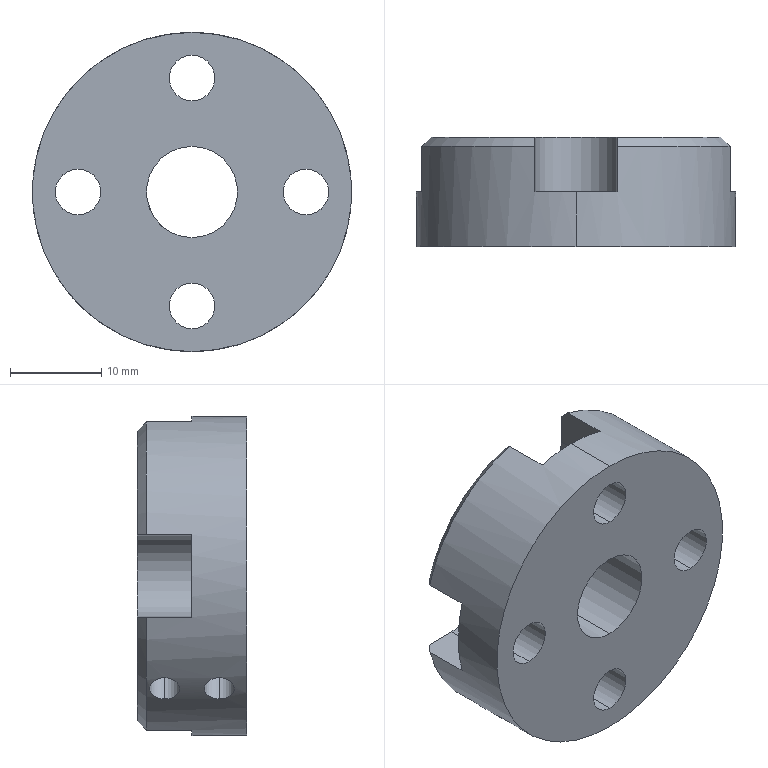Part | SolidWorks | features ICE 2, Chamfer 1, CirPattern 1, Cut 1, Extrusion 1, HoleWzd 1, RefAxis 1 | 1 solid | 39 faces | box 35 x 12 x 35 mm | volume 8080 mm3 | cylinder 21 | plane 14 | cone 4 | commonest cylinder face diameters 5 x8 9 x5 3.3 x4 10 x2 35 x2